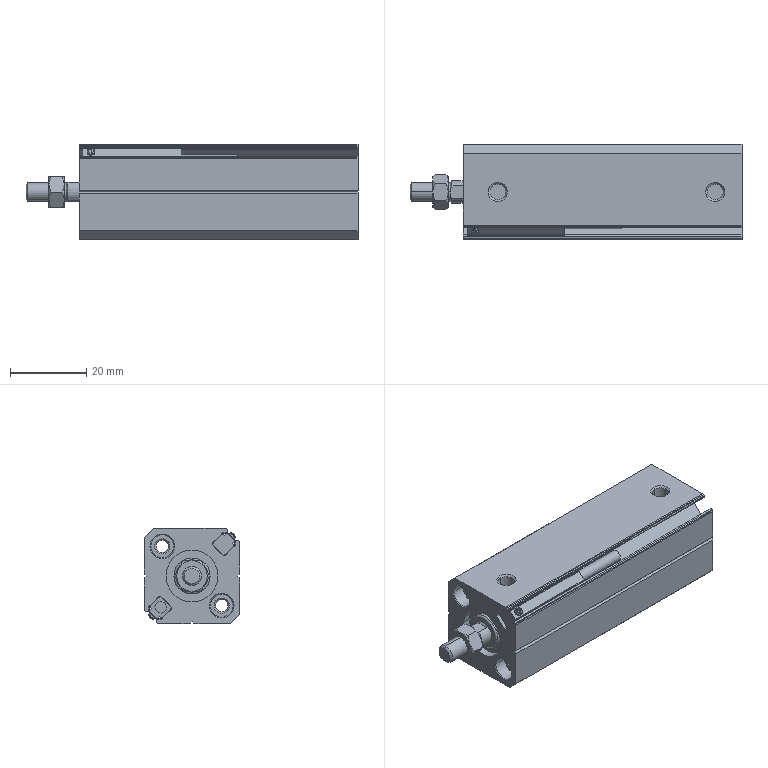Part | SolidWorks | features BaseBody 5, MoveCopyBody 2 | 5 solids | 220 faces | box 87 x 25 x 25 mm | volume 36793 mm3 | plane 90 | cylinder 76 | cone 52 | torus 2 | commonest cylinder face diameters 0.8 x19 6 x12 0.4 x9 4.134 x6 0.6 x4 1 x4